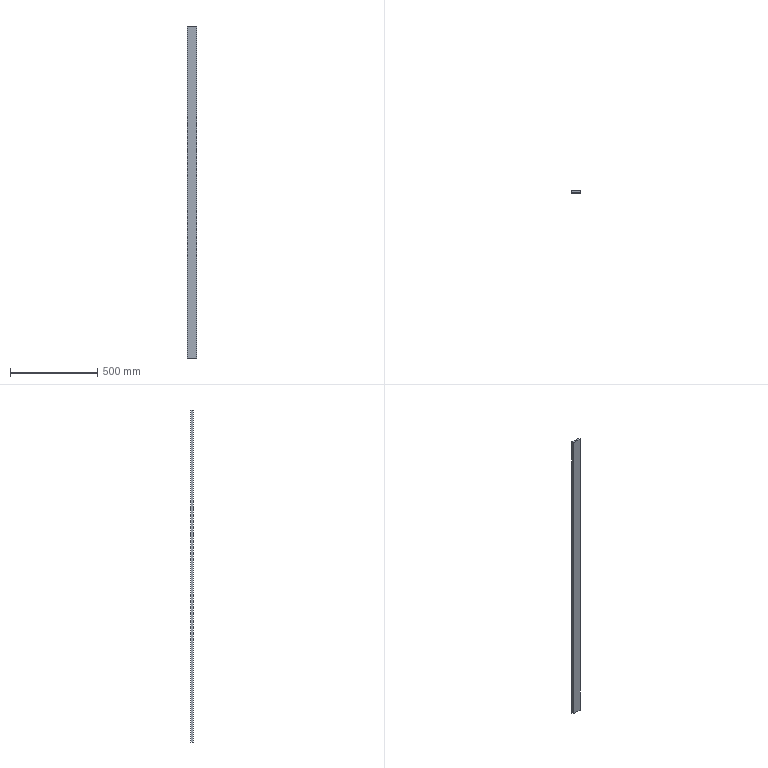Part | SolidWorks | features Extrusion 1 | 1 solid | 6 faces | box 55 x 12 x 1900 mm | volume 1254000 mm3 | plane 6
STEP:
#1=CARTESIAN_POINT('',(0.,0.,0.));
#2=VERTEX_POINT('',#1);
#3=CARTESIAN_POINT('',(0.,-12.,0.));
#4=VERTEX_POINT('',#3);
#5=CARTESIAN_POINT('',(0.,0.,0.));
#6=DIRECTION('',(0.,-1.,0.));
#7=VECTOR('',#6,1000.);
#8=LINE('',#5,#7);
#9=EDGE_CURVE('',#2,#4,#8,.T.);
#10=ORIENTED_EDGE('',*,*,#9,.T.);
#11=CARTESIAN_POINT('',(0.,-12.,1900.));
#12=VERTEX_POINT('',#11);
#13=CARTESIAN_POINT('',(0.,-12.,1900.));
#14=DIRECTION('',(0.,0.,-1.));
#15=VECTOR('',#14,1000.);
#16=LINE('',#13,#15);
#17=EDGE_CURVE('',#12,#4,#16,.T.);
#18=ORIENTED_EDGE('',*,*,#17,.F.);
#19=CARTESIAN_POINT('',(0.,0.,1900.));
#20=VERTEX_POINT('',#19);
#21=CARTESIAN_POINT('',(0.,0.,1900.));
#22=DIRECTION('',(0.,-1.,0.));
#23=VECTOR('',#22,1000.);
#24=LINE('',#21,#23);
#25=EDGE_CURVE('',#20,#12,#24,.T.);
#26=ORIENTED_EDGE('',*,*,#25,.F.);
#27=CARTESIAN_POINT('',(0.,0.,1900.));
#28=DIRECTION('',(0.,0.,-1.));
#29=VECTOR('',#28,1000.);
#30=LINE('',#27,#29);
#31=EDGE_CURVE('',#20,#2,#30,.T.);
#32=ORIENTED_EDGE('',*,*,#31,.T.);
#33=EDGE_LOOP('',(#10,#18,#26,#32));
#34=FACE_OUTER_BOUND('',#33,.T.);
#35=CARTESIAN_POINT('',(0.,0.,1900.));
#36=DIRECTION('',(1.,0.,0.));
#37=DIRECTION('',(0.,1.,0.));
#38=AXIS2_PLACEMENT_3D('',#35,#36,#37);
#39=PLANE('',#38);
#40=ADVANCED_FACE('',(#34),#39,.F.);
#41=CARTESIAN_POINT('',(55.,-12.,0.));
#42=VERTEX_POINT('',#41);
#43=CARTESIAN_POINT('',(0.,-12.,0.));
#44=DIRECTION('',(1.,0.,0.));
#45=VECTOR('',#44,1000.);
#46=LINE('',#43,#45);
#47=EDGE_CURVE('',#4,#42,#46,.T.);
#48=ORIENTED_EDGE('',*,*,#47,.T.);
#49=CARTESIAN_POINT('',(55.,-12.,1900.));
#50=VERTEX_POINT('',#49);
#51=CARTESIAN_POINT('',(55.,-12.,1900.));
#52=DIRECTION('',(0.,0.,-1.));
#53=VECTOR('',#52,1000.);
#54=LINE('',#51,#53);
#55=EDGE_CURVE('',#50,#42,#54,.T.);
#56=ORIENTED_EDGE('',*,*,#55,.F.);
#57=CARTESIAN_POINT('',(0.,-12.,1900.));
#58=DIRECTION('',(1.,0.,0.));
#59=VECTOR('',#58,1000.);
#60=LINE('',#57,#59);
#61=EDGE_CURVE('',#12,#50,#60,.T.);
#62=ORIENTED_EDGE('',*,*,#61,.F.);
#63=ORIENTED_EDGE('',*,*,#17,.T.);
#64=EDGE_LOOP('',(#48,#56,#62,#63));
#65=FACE_OUTER_BOUND('',#64,.T.);
#66=CARTESIAN_POINT('',(0.,-12.,1900.));
#67=DIRECTION('',(0.,1.,0.));
#68=DIRECTION('',(0.,0.,1.));
#69=AXIS2_PLACEMENT_3D('',#66,#67,#68);
#70=PLANE('',#69);
#71=ADVANCED_FACE('',(#65),#70,.F.);
#72=CARTESIAN_POINT('',(55.,0.,0.));
#73=VERTEX_POINT('',#72);
#74=CARTESIAN_POINT('',(55.,0.,0.));
#75=DIRECTION('',(0.,1.,0.));
#76=VECTOR('',#75,1000.);
#77=LINE('',#74,#76);
#78=EDGE_CURVE('',#42,#73,#77,.T.);
#79=ORIENTED_EDGE('',*,*,#78,.T.);
#80=CARTESIAN_POINT('',(55.,0.,1900.));
#81=VERTEX_POINT('',#80);
#82=CARTESIAN_POINT('',(55.,0.,1900.));
#83=DIRECTION('',(0.,0.,-1.));
#84=VECTOR('',#83,1000.);
#85=LINE('',#82,#84);
#86=EDGE_CURVE('',#81,#73,#85,.T.);
#87=ORIENTED_EDGE('',*,*,#86,.F.);
#88=CARTESIAN_POINT('',(55.,0.,1900.));
#89=DIRECTION('',(0.,1.,0.));
#90=VECTOR('',#89,1000.);
#91=LINE('',#88,#90);
#92=EDGE_CURVE('',#50,#81,#91,.T.);
#93=ORIENTED_EDGE('',*,*,#92,.F.);
#94=ORIENTED_EDGE('',*,*,#55,.T.);
#95=EDGE_LOOP('',(#79,#87,#93,#94));
#96=FACE_OUTER_BOUND('',#95,.T.);
#97=CARTESIAN_POINT('',(55.,0.,1900.));
#98=DIRECTION('',(-1.,0.,0.));
#99=DIRECTION('',(0.,0.,1.));
#100=AXIS2_PLACEMENT_3D('',#97,#98,#99);
#101=PLANE('',#100);
#102=ADVANCED_FACE('',(#96),#101,.F.);
#103=CARTESIAN_POINT('',(0.,0.,0.));
#104=DIRECTION('',(-1.,0.,0.));
#105=VECTOR('',#104,1000.);
#106=LINE('',#103,#105);
#107=EDGE_CURVE('',#73,#2,#106,.T.);
#108=ORIENTED_EDGE('',*,*,#107,.T.);
#109=ORIENTED_EDGE('',*,*,#31,.F.);
#110=CARTESIAN_POINT('',(0.,0.,1900.));
#111=DIRECTION('',(-1.,0.,0.));
#112=VECTOR('',#111,1000.);
#113=LINE('',#110,#112);
#114=EDGE_CURVE('',#81,#20,#113,.T.);
#115=ORIENTED_EDGE('',*,*,#114,.F.);
#116=ORIENTED_EDGE('',*,*,#86,.T.);
#117=EDGE_LOOP('',(#108,#109,#115,#116));
#118=FACE_OUTER_BOUND('',#117,.T.);
#119=CARTESIAN_POINT('',(0.,0.,1900.));
#120=DIRECTION('',(0.,-1.,0.));
#121=DIRECTION('',(0.,0.,-1.));
#122=AXIS2_PLACEMENT_3D('',#119,#120,#121);
#123=PLANE('',#122);
#124=ADVANCED_FACE('',(#118),#123,.F.);
#125=ORIENTED_EDGE('',*,*,#25,.T.);
#126=ORIENTED_EDGE('',*,*,#61,.T.);
#127=ORIENTED_EDGE('',*,*,#92,.T.);
#128=ORIENTED_EDGE('',*,*,#114,.T.);
#129=EDGE_LOOP('',(#125,#126,#127,#128));
#130=FACE_OUTER_BOUND('',#129,.T.);
#131=CARTESIAN_POINT('',(0.,0.,1900.));
#132=DIRECTION('',(0.,0.,1.));
#133=DIRECTION('',(1.,0.,0.));
#134=AXIS2_PLACEMENT_3D('',#131,#132,#133);
#135=PLANE('',#134);
#136=ADVANCED_FACE('',(#130),#135,.T.);
#137=ORIENTED_EDGE('',*,*,#9,.F.);
#138=ORIENTED_EDGE('',*,*,#107,.F.);
#139=ORIENTED_EDGE('',*,*,#78,.F.);
#140=ORIENTED_EDGE('',*,*,#47,.F.);
#141=EDGE_LOOP('',(#137,#138,#139,#140));
#142=FACE_OUTER_BOUND('',#141,.T.);
#143=CARTESIAN_POINT('',(0.,0.,0.));
#144=DIRECTION('',(0.,0.,1.));
#145=DIRECTION('',(1.,0.,0.));
#146=AXIS2_PLACEMENT_3D('',#143,#144,#145);
#147=PLANE('',#146);
#148=ADVANCED_FACE('',(#142),#147,.F.);
#149=CLOSED_SHELL('',(#40,#71,#102,#124,#136,#148));
#150=MANIFOLD_SOLID_BREP('',#149);
#151=CARTESIAN_POINT('',(0.,0.,0.));
#152=DIRECTION('',(0.,0.,1.));
#153=DIRECTION('',(1.,0.,0.));
#154=AXIS2_PLACEMENT_3D('',#151,#152,#153);
#155=(LENGTH_UNIT()NAMED_UNIT(*)SI_UNIT(.MILLI.,.METRE.));
#156=UNCERTAINTY_MEASURE_WITH_UNIT(LENGTH_MEASURE(0.00001),#155,'','');
#157=(NAMED_UNIT(*)PLANE_ANGLE_UNIT()SI_UNIT($,.RADIAN.));
#158=(NAMED_UNIT(*)SI_UNIT($,.STERADIAN.)SOLID_ANGLE_UNIT());
#159=(GEOMETRIC_REPRESENTATION_CONTEXT(3)GLOBAL_UNCERTAINTY_ASSIGNED_CONTEXT((#156))GLOBAL_UNIT_ASSIGNED_CONTEXT((#155,#157,#158))REPRESENTATION_CONTEXT('',''));
#160=ADVANCED_BREP_SHAPE_REPRESENTATION('',(#150,#154),#159);